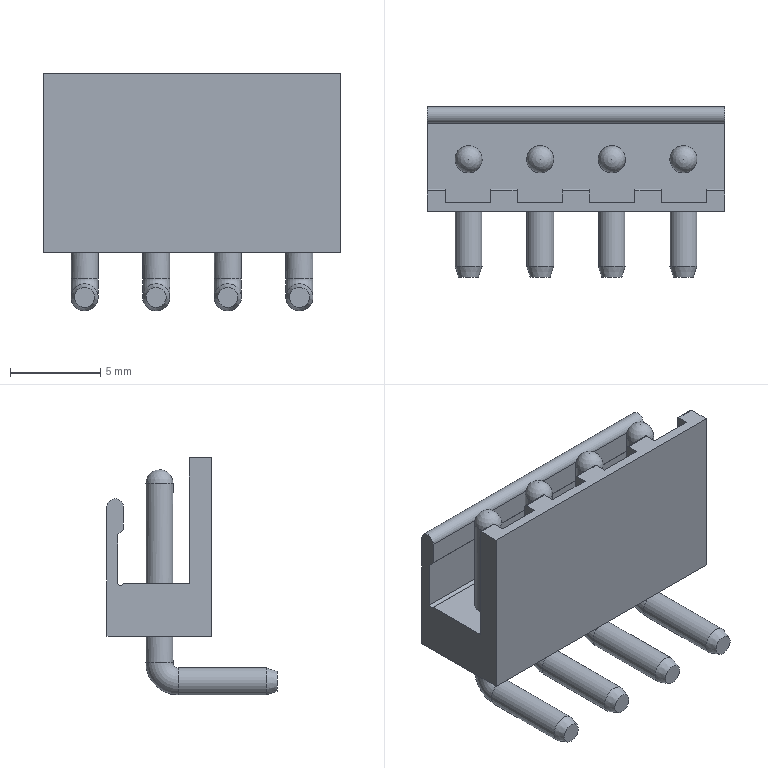Part | STEP file | JL27-04ZJW | 1 solid | 62 faces | box 16.44 x 9.4 x 13.15 mm | volume 524.314 mm3 | plane 31 | cylinder 19 | torus 4 | sphere 4 | cone 4 | commonest cylinder face diameters 1.5 x12 0.2 x5 0.337 x1 0.9 x1